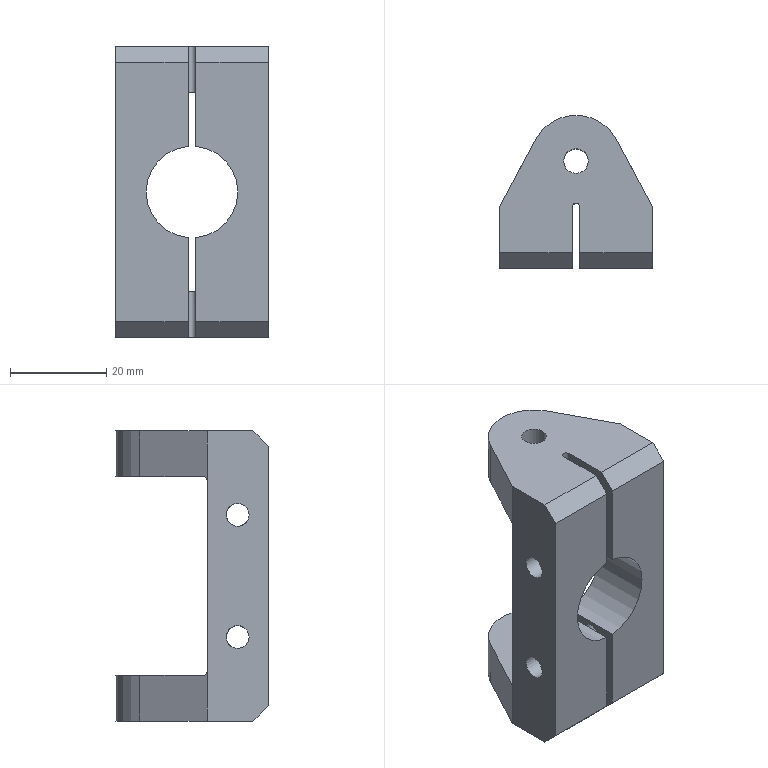Part | NX | features MG0330 trunion parts 24(stanchion group) 2 | 1 solid | 38 faces | box 31.75 x 31.75 x 60.325 mm | volume 25721 mm3 | plane 22 | cylinder 16 | commonest cylinder face diameters 1.524 x4 4.763 x4 19.05 x4 1.587 x2 5.105 x2
STEP:
#1=CARTESIAN_POINT('',(15.469,-15.113,-20.637));
#2=VERTEX_POINT('',#1);
#3=CARTESIAN_POINT('',(15.875,-15.875,-19.875));
#4=VERTEX_POINT('',#3);
#5=CARTESIAN_POINT('',(15.469,-15.113,-19.875));
#6=DIRECTION('',(0.8824,0.4706,0.));
#7=DIRECTION('',(0.4706,-0.8824,0.));
#8=AXIS2_PLACEMENT_3D('',#5,#6,#7);
#9=ELLIPSE('',#8,0.8636,0.762);
#10=EDGE_CURVE('',#2,#4,#9,.F.);
#11=ORIENTED_EDGE('',*,*,#10,.F.);
#12=CARTESIAN_POINT('',(0.2222,-15.113,-20.637));
#13=VERTEX_POINT('',#12);
#14=CARTESIAN_POINT('',(15.875,-15.113,-20.637));
#15=DIRECTION('',(-1.,0.,0.));
#16=VECTOR('',#15,1000.);
#17=LINE('',#14,#16);
#18=EDGE_CURVE('',#13,#2,#17,.F.);
#19=ORIENTED_EDGE('',*,*,#18,.F.);
#20=CARTESIAN_POINT('',(0.7937,-15.875,-19.875));
#21=VERTEX_POINT('',#20);
#22=CARTESIAN_POINT('',(0.2222,-15.113,-20.637));
#23=CARTESIAN_POINT('',(0.4532,-15.18,-20.637));
#24=CARTESIAN_POINT('',(0.8336,-15.592,-20.608));
#25=CARTESIAN_POINT('',(0.7937,-15.875,-20.117));
#26=CARTESIAN_POINT('',(0.7937,-15.875,-19.875));
#27=B_SPLINE_CURVE_WITH_KNOTS('',3,(#22,#23,#24,#25,#26),.UNSPECIFIED.,.F.,.F.,(4,1,4),(0.0004486,0.001169,0.001889),.UNSPECIFIED.);
#28=EDGE_CURVE('',#13,#21,#27,.T.);
#29=ORIENTED_EDGE('',*,*,#28,.T.);
#30=CARTESIAN_POINT('',(-15.875,-15.875,-19.875));
#31=DIRECTION('',(-1.,0.,0.));
#32=VECTOR('',#31,1000.);
#33=LINE('',#30,#32);
#34=EDGE_CURVE('',#4,#21,#33,.T.);
#35=ORIENTED_EDGE('',*,*,#34,.F.);
#36=EDGE_LOOP('',(#11,#19,#29,#35));
#37=FACE_BOUND('',#36,.T.);
#38=CARTESIAN_POINT('',(15.875,-15.113,-19.875));
#39=DIRECTION('',(1.,0.,0.));
#40=DIRECTION('',(0.,0.,-1.));
#41=AXIS2_PLACEMENT_3D('',#38,#39,#40);
#42=CYLINDRICAL_SURFACE('',#41,0.762);
#43=ADVANCED_FACE('',(#37),#42,.F.);
#44=CARTESIAN_POINT('',(0.,-8.903,-30.163));
#45=VERTEX_POINT('',#44);
#46=CARTESIAN_POINT('',(0.,-6.35,-30.163));
#47=DIRECTION('',(0.,0.,1.));
#48=DIRECTION('',(0.,-1.,0.));
#49=AXIS2_PLACEMENT_3D('',#46,#47,#48);
#50=CIRCLE('',#49,2.553);
#51=EDGE_CURVE('',#45,#45,#50,.T.);
#52=ORIENTED_EDGE('',*,*,#51,.T.);
#53=EDGE_LOOP('',(#52));
#54=FACE_BOUND('',#53,.T.);
#55=CARTESIAN_POINT('',(-8.404,-1.868,-30.163));
#56=VERTEX_POINT('',#55);
#57=CARTESIAN_POINT('',(-15.875,-15.875,-30.163));
#58=VERTEX_POINT('',#57);
#59=CARTESIAN_POINT('',(-0.9338,12.14,-30.163));
#60=DIRECTION('',(-0.4706,-0.8824,0.));
#61=VECTOR('',#60,1000.);
#62=LINE('',#59,#61);
#63=EDGE_CURVE('',#56,#58,#62,.T.);
#64=ORIENTED_EDGE('',*,*,#63,.F.);
#65=CARTESIAN_POINT('',(8.404,-1.868,-30.163));
#66=VERTEX_POINT('',#65);
#67=CARTESIAN_POINT('',(0.,-6.35,-30.163));
#68=DIRECTION('',(0.,0.,1.));
#69=DIRECTION('',(0.,-1.,0.));
#70=AXIS2_PLACEMENT_3D('',#67,#68,#69);
#71=CIRCLE('',#70,9.525);
#72=EDGE_CURVE('',#66,#56,#71,.T.);
#73=ORIENTED_EDGE('',*,*,#72,.F.);
#74=CARTESIAN_POINT('',(15.875,-15.875,-30.163));
#75=VERTEX_POINT('',#74);
#76=CARTESIAN_POINT('',(7.965,-1.044,-30.163));
#77=DIRECTION('',(-0.4706,0.8824,0.));
#78=VECTOR('',#77,1000.);
#79=LINE('',#76,#78);
#80=EDGE_CURVE('',#75,#66,#79,.T.);
#81=ORIENTED_EDGE('',*,*,#80,.F.);
#82=CARTESIAN_POINT('',(15.875,-25.4,-30.163));
#83=VERTEX_POINT('',#82);
#84=CARTESIAN_POINT('',(15.875,3.175,-30.163));
#85=DIRECTION('',(0.,1.,0.));
#86=VECTOR('',#85,1000.);
#87=LINE('',#84,#86);
#88=EDGE_CURVE('',#83,#75,#87,.T.);
#89=ORIENTED_EDGE('',*,*,#88,.F.);
#90=CARTESIAN_POINT('',(0.7937,-25.4,-30.163));
#91=VERTEX_POINT('',#90);
#92=CARTESIAN_POINT('',(15.875,-25.4,-30.163));
#93=DIRECTION('',(-1.,0.,0.));
#94=VECTOR('',#93,1000.);
#95=LINE('',#92,#94);
#96=EDGE_CURVE('',#83,#91,#95,.T.);
#97=ORIENTED_EDGE('',*,*,#96,.T.);
#98=CARTESIAN_POINT('',(0.7937,-15.875,-30.163));
#99=VERTEX_POINT('',#98);
#100=CARTESIAN_POINT('',(0.7937,3.175,-30.163));
#101=DIRECTION('',(0.,1.,0.));
#102=VECTOR('',#101,1000.);
#103=LINE('',#100,#102);
#104=EDGE_CURVE('',#91,#99,#103,.T.);
#105=ORIENTED_EDGE('',*,*,#104,.T.);
#106=CARTESIAN_POINT('',(-0.7937,-15.875,-30.163));
#107=VERTEX_POINT('',#106);
#108=CARTESIAN_POINT('',(0.,-15.875,-30.163));
#109=DIRECTION('',(0.,0.,1.));
#110=DIRECTION('',(0.,-1.,0.));
#111=AXIS2_PLACEMENT_3D('',#108,#109,#110);
#112=CIRCLE('',#111,0.7937);
#113=EDGE_CURVE('',#99,#107,#112,.T.);
#114=ORIENTED_EDGE('',*,*,#113,.T.);
#115=CARTESIAN_POINT('',(-0.7937,-25.4,-30.163));
#116=VERTEX_POINT('',#115);
#117=CARTESIAN_POINT('',(-0.7937,3.175,-30.163));
#118=DIRECTION('',(0.,-1.,0.));
#119=VECTOR('',#118,1000.);
#120=LINE('',#117,#119);
#121=EDGE_CURVE('',#107,#116,#120,.T.);
#122=ORIENTED_EDGE('',*,*,#121,.T.);
#123=CARTESIAN_POINT('',(-15.875,-25.4,-30.163));
#124=VERTEX_POINT('',#123);
#125=CARTESIAN_POINT('',(15.875,-25.4,-30.163));
#126=DIRECTION('',(-1.,0.,0.));
#127=VECTOR('',#126,1000.);
#128=LINE('',#125,#127);
#129=EDGE_CURVE('',#116,#124,#128,.T.);
#130=ORIENTED_EDGE('',*,*,#129,.T.);
#131=CARTESIAN_POINT('',(-15.875,3.175,-30.163));
#132=DIRECTION('',(0.,1.,0.));
#133=VECTOR('',#132,1000.);
#134=LINE('',#131,#133);
#135=EDGE_CURVE('',#124,#58,#134,.T.);
#136=ORIENTED_EDGE('',*,*,#135,.T.);
#137=EDGE_LOOP('',(#64,#73,#81,#89,#97,#105,#114,#122,#130,#136));
#138=FACE_BOUND('',#137,.T.);
#139=CARTESIAN_POINT('',(15.875,3.175,-30.163));
#140=DIRECTION('',(0.,0.,1.));
#141=DIRECTION('',(0.,-1.,0.));
#142=AXIS2_PLACEMENT_3D('',#139,#140,#141);
#143=PLANE('',#142);
#144=ADVANCED_FACE('',(#54,#138),#143,.F.);
#145=CARTESIAN_POINT('',(0.,-3.797,-20.637));
#146=VERTEX_POINT('',#145);
#147=CARTESIAN_POINT('',(0.,-6.35,-20.637));
#148=DIRECTION('',(0.,0.,-1.));
#149=DIRECTION('',(0.,1.,0.));
#150=AXIS2_PLACEMENT_3D('',#147,#148,#149);
#151=CIRCLE('',#150,2.553);
#152=EDGE_CURVE('',#146,#146,#151,.T.);
#153=ORIENTED_EDGE('',*,*,#152,.T.);
#154=EDGE_LOOP('',(#153));
#155=FACE_BOUND('',#154,.T.);
#156=CARTESIAN_POINT('',(-15.469,-15.113,-20.637));
#157=VERTEX_POINT('',#156);
#158=CARTESIAN_POINT('',(-8.404,-1.868,-20.637));
#159=VERTEX_POINT('',#158);
#160=CARTESIAN_POINT('',(-0.9338,12.14,-20.637));
#161=DIRECTION('',(0.4706,0.8824,0.));
#162=VECTOR('',#161,1000.);
#163=LINE('',#160,#162);
#164=EDGE_CURVE('',#157,#159,#163,.T.);
#165=ORIENTED_EDGE('',*,*,#164,.F.);
#166=CARTESIAN_POINT('',(-0.2222,-15.113,-20.637));
#167=VERTEX_POINT('',#166);
#168=CARTESIAN_POINT('',(15.875,-15.113,-20.637));
#169=DIRECTION('',(-1.,0.,0.));
#170=VECTOR('',#169,1000.);
#171=LINE('',#168,#170);
#172=EDGE_CURVE('',#157,#167,#171,.F.);
#173=ORIENTED_EDGE('',*,*,#172,.T.);
#174=CARTESIAN_POINT('',(0.,-15.875,-20.637));
#175=DIRECTION('',(0.,0.,-1.));
#176=DIRECTION('',(0.,1.,0.));
#177=AXIS2_PLACEMENT_3D('',#174,#175,#176);
#178=CIRCLE('',#177,0.7937);
#179=EDGE_CURVE('',#167,#13,#178,.T.);
#180=ORIENTED_EDGE('',*,*,#179,.T.);
#181=ORIENTED_EDGE('',*,*,#18,.T.);
#182=CARTESIAN_POINT('',(8.404,-1.868,-20.637));
#183=VERTEX_POINT('',#182);
#184=CARTESIAN_POINT('',(7.965,-1.044,-20.637));
#185=DIRECTION('',(0.4706,-0.8824,0.));
#186=VECTOR('',#185,1000.);
#187=LINE('',#184,#186);
#188=EDGE_CURVE('',#183,#2,#187,.T.);
#189=ORIENTED_EDGE('',*,*,#188,.F.);
#190=CARTESIAN_POINT('',(0.,-6.35,-20.637));
#191=DIRECTION('',(0.,0.,-1.));
#192=DIRECTION('',(0.,1.,0.));
#193=AXIS2_PLACEMENT_3D('',#190,#191,#192);
#194=CIRCLE('',#193,9.525);
#195=EDGE_CURVE('',#159,#183,#194,.T.);
#196=ORIENTED_EDGE('',*,*,#195,.F.);
#197=EDGE_LOOP('',(#165,#173,#180,#181,#189,#196));
#198=FACE_BOUND('',#197,.T.);
#199=CARTESIAN_POINT('',(15.875,3.175,-20.637));
#200=DIRECTION('',(0.,0.,-1.));
#201=DIRECTION('',(0.,1.,0.));
#202=AXIS2_PLACEMENT_3D('',#199,#200,#201);
#203=PLANE('',#202);
#204=ADVANCED_FACE('',(#155,#198),#203,.F.);
#205=CARTESIAN_POINT('',(15.875,-22.225,15.081));
#206=VERTEX_POINT('',#205);
#207=CARTESIAN_POINT('',(15.875,-22.225,12.7));
#208=DIRECTION('',(-1.,0.,0.));
#209=DIRECTION('',(0.,0.,1.));
#210=AXIS2_PLACEMENT_3D('',#207,#208,#209);
#211=CIRCLE('',#210,2.381);
#212=EDGE_CURVE('',#206,#206,#211,.T.);
#213=ORIENTED_EDGE('',*,*,#212,.T.);
#214=EDGE_LOOP('',(#213));
#215=FACE_BOUND('',#214,.T.);
#216=CARTESIAN_POINT('',(15.875,-22.225,-10.319));
#217=VERTEX_POINT('',#216);
#218=CARTESIAN_POINT('',(15.875,-22.225,-12.7));
#219=DIRECTION('',(-1.,0.,0.));
#220=DIRECTION('',(0.,0.,1.));
#221=AXIS2_PLACEMENT_3D('',#218,#219,#220);
#222=CIRCLE('',#221,2.381);
#223=EDGE_CURVE('',#217,#217,#222,.T.);
#224=ORIENTED_EDGE('',*,*,#223,.T.);
#225=EDGE_LOOP('',(#224));
#226=FACE_BOUND('',#225,.T.);
#227=CARTESIAN_POINT('',(15.875,-15.875,30.163));
#228=VERTEX_POINT('',#227);
#229=CARTESIAN_POINT('',(15.875,-15.875,19.875));
#230=VERTEX_POINT('',#229);
#231=CARTESIAN_POINT('',(15.875,-15.875,494.417));
#232=DIRECTION('',(0.,0.,-1.));
#233=VECTOR('',#232,1000.);
#234=LINE('',#231,#233);
#235=EDGE_CURVE('',#228,#230,#234,.T.);
#236=ORIENTED_EDGE('',*,*,#235,.F.);
#237=CARTESIAN_POINT('',(15.875,-25.4,30.163));
#238=VERTEX_POINT('',#237);
#239=CARTESIAN_POINT('',(15.875,3.175,30.163));
#240=DIRECTION('',(0.,1.,0.));
#241=VECTOR('',#240,1000.);
#242=LINE('',#239,#241);
#243=EDGE_CURVE('',#238,#228,#242,.T.);
#244=ORIENTED_EDGE('',*,*,#243,.F.);
#245=CARTESIAN_POINT('',(15.875,-28.575,26.988));
#246=VERTEX_POINT('',#245);
#247=CARTESIAN_POINT('',(15.875,-25.4,30.163));
#248=DIRECTION('',(0.,-0.7071,-0.7071));
#249=VECTOR('',#248,1000.);
#250=LINE('',#247,#249);
#251=EDGE_CURVE('',#246,#238,#250,.F.);
#252=ORIENTED_EDGE('',*,*,#251,.F.);
#253=CARTESIAN_POINT('',(15.875,-28.575,-26.988));
#254=VERTEX_POINT('',#253);
#255=CARTESIAN_POINT('',(15.875,-28.575,-30.163));
#256=DIRECTION('',(0.,0.,-1.));
#257=VECTOR('',#256,1000.);
#258=LINE('',#255,#257);
#259=EDGE_CURVE('',#246,#254,#258,.T.);
#260=ORIENTED_EDGE('',*,*,#259,.T.);
#261=CARTESIAN_POINT('',(15.875,-25.4,-30.163));
#262=DIRECTION('',(0.,-0.7071,0.7071));
#263=VECTOR('',#262,1000.);
#264=LINE('',#261,#263);
#265=EDGE_CURVE('',#254,#83,#264,.F.);
#266=ORIENTED_EDGE('',*,*,#265,.T.);
#267=ORIENTED_EDGE('',*,*,#88,.T.);
#268=CARTESIAN_POINT('',(15.875,-15.875,494.417));
#269=DIRECTION('',(0.,0.,-1.));
#270=VECTOR('',#269,1000.);
#271=LINE('',#268,#270);
#272=EDGE_CURVE('',#4,#75,#271,.T.);
#273=ORIENTED_EDGE('',*,*,#272,.F.);
#274=CARTESIAN_POINT('',(15.875,-15.875,-20.637));
#275=DIRECTION('',(0.,0.,1.));
#276=VECTOR('',#275,1000.);
#277=LINE('',#274,#276);
#278=EDGE_CURVE('',#4,#230,#277,.T.);
#279=ORIENTED_EDGE('',*,*,#278,.T.);
#280=EDGE_LOOP('',(#236,#244,#252,#260,#266,#267,#273,#279));
#281=FACE_BOUND('',#280,.T.);
#282=CARTESIAN_POINT('',(15.875,-28.575,-30.163));
#283=DIRECTION('',(-1.,0.,0.));
#284=DIRECTION('',(0.,0.,1.));
#285=AXIS2_PLACEMENT_3D('',#282,#283,#284);
#286=PLANE('',#285);
#287=ADVANCED_FACE('',(#215,#226,#281),#286,.F.);
#288=CARTESIAN_POINT('',(-15.875,-22.225,15.081));
#289=VERTEX_POINT('',#288);
#290=CARTESIAN_POINT('',(-15.875,-22.225,12.7));
#291=DIRECTION('',(-1.,0.,0.));
#292=DIRECTION('',(0.,0.,1.));
#293=AXIS2_PLACEMENT_3D('',#290,#291,#292);
#294=CIRCLE('',#293,2.381);
#295=EDGE_CURVE('',#289,#289,#294,.F.);
#296=ORIENTED_EDGE('',*,*,#295,.T.);
#297=EDGE_LOOP('',(#296));
#298=FACE_BOUND('',#297,.T.);
#299=CARTESIAN_POINT('',(-15.875,-22.225,-10.319));
#300=VERTEX_POINT('',#299);
#301=CARTESIAN_POINT('',(-15.875,-22.225,-12.7));
#302=DIRECTION('',(-1.,0.,0.));
#303=DIRECTION('',(0.,0.,1.));
#304=AXIS2_PLACEMENT_3D('',#301,#302,#303);
#305=CIRCLE('',#304,2.381);
#306=EDGE_CURVE('',#300,#300,#305,.F.);
#307=ORIENTED_EDGE('',*,*,#306,.T.);
#308=EDGE_LOOP('',(#307));
#309=FACE_BOUND('',#308,.T.);
#310=CARTESIAN_POINT('',(-15.875,-25.4,30.163));
#311=VERTEX_POINT('',#310);
#312=CARTESIAN_POINT('',(-15.875,-15.875,30.163));
#313=VERTEX_POINT('',#312);
#314=CARTESIAN_POINT('',(-15.875,3.175,30.163));
#315=DIRECTION('',(0.,1.,0.));
#316=VECTOR('',#315,1000.);
#317=LINE('',#314,#316);
#318=EDGE_CURVE('',#311,#313,#317,.T.);
#319=ORIENTED_EDGE('',*,*,#318,.T.);
#320=CARTESIAN_POINT('',(-15.875,-15.875,19.875));
#321=VERTEX_POINT('',#320);
#322=CARTESIAN_POINT('',(-15.875,-15.875,494.417));
#323=DIRECTION('',(0.,0.,-1.));
#324=VECTOR('',#323,1000.);
#325=LINE('',#322,#324);
#326=EDGE_CURVE('',#313,#321,#325,.T.);
#327=ORIENTED_EDGE('',*,*,#326,.T.);
#328=CARTESIAN_POINT('',(-15.875,-15.875,-19.875));
#329=VERTEX_POINT('',#328);
#330=CARTESIAN_POINT('',(-15.875,-15.875,-20.637));
#331=DIRECTION('',(0.,0.,1.));
#332=VECTOR('',#331,1000.);
#333=LINE('',#330,#332);
#334=EDGE_CURVE('',#329,#321,#333,.T.);
#335=ORIENTED_EDGE('',*,*,#334,.F.);
#336=CARTESIAN_POINT('',(-15.875,-15.875,494.417));
#337=DIRECTION('',(0.,0.,-1.));
#338=VECTOR('',#337,1000.);
#339=LINE('',#336,#338);
#340=EDGE_CURVE('',#329,#58,#339,.T.);
#341=ORIENTED_EDGE('',*,*,#340,.T.);
#342=ORIENTED_EDGE('',*,*,#135,.F.);
#343=CARTESIAN_POINT('',(-15.875,-28.575,-26.988));
#344=VERTEX_POINT('',#343);
#345=CARTESIAN_POINT('',(-15.875,-26.988,-28.575));
#346=DIRECTION('',(0.,0.7071,-0.7071));
#347=VECTOR('',#346,1000.);
#348=LINE('',#345,#347);
#349=EDGE_CURVE('',#124,#344,#348,.F.);
#350=ORIENTED_EDGE('',*,*,#349,.T.);
#351=CARTESIAN_POINT('',(-15.875,-28.575,26.988));
#352=VERTEX_POINT('',#351);
#353=CARTESIAN_POINT('',(-15.875,-28.575,-30.163));
#354=DIRECTION('',(0.,0.,-1.));
#355=VECTOR('',#354,1000.);
#356=LINE('',#353,#355);
#357=EDGE_CURVE('',#352,#344,#356,.T.);
#358=ORIENTED_EDGE('',*,*,#357,.F.);
#359=CARTESIAN_POINT('',(-15.875,-26.988,28.575));
#360=DIRECTION('',(0.,0.7071,0.7071));
#361=VECTOR('',#360,1000.);
#362=LINE('',#359,#361);
#363=EDGE_CURVE('',#311,#352,#362,.F.);
#364=ORIENTED_EDGE('',*,*,#363,.F.);
#365=EDGE_LOOP('',(#319,#327,#335,#341,#342,#350,#358,#364));
#366=FACE_BOUND('',#365,.T.);
#367=CARTESIAN_POINT('',(-15.875,-28.575,-30.163));
#368=DIRECTION('',(-1.,0.,0.));
#369=DIRECTION('',(0.,0.,1.));
#370=AXIS2_PLACEMENT_3D('',#367,#368,#369);
#371=PLANE('',#370);
#372=ADVANCED_FACE('',(#298,#309,#366),#371,.T.);
#373=CARTESIAN_POINT('',(-15.469,-15.113,-19.875));
#374=DIRECTION('',(-0.8824,0.4706,0.));
#375=DIRECTION('',(0.4706,0.8824,0.));
#376=AXIS2_PLACEMENT_3D('',#373,#374,#375);
#377=ELLIPSE('',#376,0.8636,0.762);
#378=EDGE_CURVE('',#329,#157,#377,.F.);
#379=ORIENTED_EDGE('',*,*,#378,.F.);
#380=CARTESIAN_POINT('',(-0.7937,-15.875,-19.875));
#381=VERTEX_POINT('',#380);
#382=CARTESIAN_POINT('',(-15.875,-15.875,-19.875));
#383=DIRECTION('',(-1.,0.,0.));
#384=VECTOR('',#383,1000.);
#385=LINE('',#382,#384);
#386=EDGE_CURVE('',#381,#329,#385,.T.);
#387=ORIENTED_EDGE('',*,*,#386,.F.);
#388=CARTESIAN_POINT('',(-0.7938,-15.875,-19.875));
#389=CARTESIAN_POINT('',(-0.7938,-15.875,-20.118));
#390=CARTESIAN_POINT('',(-0.834,-15.595,-20.605));
#391=CARTESIAN_POINT('',(-0.4553,-15.181,-20.637));
#392=CARTESIAN_POINT('',(-0.2222,-15.113,-20.637));
#393=B_SPLINE_CURVE_WITH_KNOTS('',3,(#388,#389,#390,#391,#392),.UNSPECIFIED.,.F.,.F.,(4,1,4),(0.005213,0.005931,0.006649),.UNSPECIFIED.);
#394=EDGE_CURVE('',#381,#167,#393,.T.);
#395=ORIENTED_EDGE('',*,*,#394,.T.);
#396=ORIENTED_EDGE('',*,*,#172,.F.);
#397=EDGE_LOOP('',(#379,#387,#395,#396));
#398=FACE_BOUND('',#397,.T.);
#399=CARTESIAN_POINT('',(15.875,-15.113,-19.875));
#400=DIRECTION('',(1.,0.,0.));
#401=DIRECTION('',(0.,0.,-1.));
#402=AXIS2_PLACEMENT_3D('',#399,#400,#401);
#403=CYLINDRICAL_SURFACE('',#402,0.762);
#404=ADVANCED_FACE('',(#398),#403,.F.);
#405=CARTESIAN_POINT('',(15.469,-15.113,20.637));
#406=VERTEX_POINT('',#405);
#407=CARTESIAN_POINT('',(15.469,-15.113,19.875));
#408=DIRECTION('',(0.8824,0.4706,0.));
#409=DIRECTION('',(0.4706,-0.8824,0.));
#410=AXIS2_PLACEMENT_3D('',#407,#408,#409);
#411=ELLIPSE('',#410,0.8636,0.762);
#412=EDGE_CURVE('',#230,#406,#411,.F.);
#413=ORIENTED_EDGE('',*,*,#412,.F.);
#414=CARTESIAN_POINT('',(0.7937,-15.875,19.875));
#415=VERTEX_POINT('',#414);
#416=CARTESIAN_POINT('',(-15.875,-15.875,19.875));
#417=DIRECTION('',(-1.,0.,0.));
#418=VECTOR('',#417,1000.);
#419=LINE('',#416,#418);
#420=EDGE_CURVE('',#230,#415,#419,.T.);
#421=ORIENTED_EDGE('',*,*,#420,.T.);
#422=CARTESIAN_POINT('',(0.2222,-15.113,20.637));
#423=VERTEX_POINT('',#422);
#424=CARTESIAN_POINT('',(0.2222,-15.113,20.637));
#425=CARTESIAN_POINT('',(0.4532,-15.18,20.637));
#426=CARTESIAN_POINT('',(0.8336,-15.592,20.608));
#427=CARTESIAN_POINT('',(0.7937,-15.875,20.117));
#428=CARTESIAN_POINT('',(0.7937,-15.875,19.875));
#429=B_SPLINE_CURVE_WITH_KNOTS('',3,(#424,#425,#426,#427,#428),.UNSPECIFIED.,.F.,.F.,(4,1,4),(0.0004486,0.001169,0.001889),.UNSPECIFIED.);
#430=EDGE_CURVE('',#423,#415,#429,.T.);
#431=ORIENTED_EDGE('',*,*,#430,.F.);
#432=CARTESIAN_POINT('',(15.875,-15.113,20.637));
#433=DIRECTION('',(-1.,0.,0.));
#434=VECTOR('',#433,1000.);
#435=LINE('',#432,#434);
#436=EDGE_CURVE('',#423,#406,#435,.F.);
#437=ORIENTED_EDGE('',*,*,#436,.T.);
#438=EDGE_LOOP('',(#413,#421,#431,#437));
#439=FACE_BOUND('',#438,.T.);
#440=CARTESIAN_POINT('',(15.875,-15.113,19.875));
#441=DIRECTION('',(1.,0.,0.));
#442=DIRECTION('',(0.,0.,1.));
#443=AXIS2_PLACEMENT_3D('',#440,#441,#442);
#444=CYLINDRICAL_SURFACE('',#443,0.762);
#445=ADVANCED_FACE('',(#439),#444,.F.);
#446=CARTESIAN_POINT('',(0.,-3.797,30.163));
#447=VERTEX_POINT('',#446);
#448=CARTESIAN_POINT('',(0.,-6.35,30.163));
#449=DIRECTION('',(0.,0.,-1.));
#450=DIRECTION('',(0.,1.,0.));
#451=AXIS2_PLACEMENT_3D('',#448,#449,#450);
#452=CIRCLE('',#451,2.553);
#453=EDGE_CURVE('',#447,#447,#452,.F.);
#454=ORIENTED_EDGE('',*,*,#453,.F.);
#455=EDGE_LOOP('',(#454));
#456=FACE_BOUND('',#455,.T.);
#457=CARTESIAN_POINT('',(-8.404,-1.868,30.163));
#458=VERTEX_POINT('',#457);
#459=CARTESIAN_POINT('',(-0.9338,12.14,30.163));
#460=DIRECTION('',(0.4706,0.8824,0.));
#461=VECTOR('',#460,1000.);
#462=LINE('',#459,#461);
#463=EDGE_CURVE('',#313,#458,#462,.T.);
#464=ORIENTED_EDGE('',*,*,#463,.F.);
#465=ORIENTED_EDGE('',*,*,#318,.F.);
#466=CARTESIAN_POINT('',(-0.7937,-25.4,30.163));
#467=VERTEX_POINT('',#466);
#468=CARTESIAN_POINT('',(15.875,-25.4,30.163));
#469=DIRECTION('',(-1.,0.,0.));
#470=VECTOR('',#469,1000.);
#471=LINE('',#468,#470);
#472=EDGE_CURVE('',#467,#311,#471,.T.);
#473=ORIENTED_EDGE('',*,*,#472,.F.);
#474=CARTESIAN_POINT('',(-0.7937,-15.875,30.163));
#475=VERTEX_POINT('',#474);
#476=CARTESIAN_POINT('',(-0.7937,3.175,30.163));
#477=DIRECTION('',(0.,-1.,0.));
#478=VECTOR('',#477,1000.);
#479=LINE('',#476,#478);
#480=EDGE_CURVE('',#475,#467,#479,.T.);
#481=ORIENTED_EDGE('',*,*,#480,.F.);
#482=CARTESIAN_POINT('',(0.7937,-15.875,30.163));
#483=VERTEX_POINT('',#482);
#484=CARTESIAN_POINT('',(0.,-15.875,30.163));
#485=DIRECTION('',(0.,0.,1.));
#486=DIRECTION('',(0.,-1.,0.));
#487=AXIS2_PLACEMENT_3D('',#484,#485,#486);
#488=CIRCLE('',#487,0.7937);
#489=EDGE_CURVE('',#483,#475,#488,.T.);
#490=ORIENTED_EDGE('',*,*,#489,.F.);
#491=CARTESIAN_POINT('',(0.7937,-25.4,30.163));
#492=VERTEX_POINT('',#491);
#493=CARTESIAN_POINT('',(0.7937,3.175,30.163));
#494=DIRECTION('',(0.,1.,0.));
#495=VECTOR('',#494,1000.);
#496=LINE('',#493,#495);
#497=EDGE_CURVE('',#492,#483,#496,.T.);
#498=ORIENTED_EDGE('',*,*,#497,.F.);
#499=CARTESIAN_POINT('',(15.875,-25.4,30.163));
#500=DIRECTION('',(-1.,0.,0.));
#501=VECTOR('',#500,1000.);
#502=LINE('',#499,#501);
#503=EDGE_CURVE('',#238,#492,#502,.T.);
#504=ORIENTED_EDGE('',*,*,#503,.F.);
#505=ORIENTED_EDGE('',*,*,#243,.T.);
#506=CARTESIAN_POINT('',(8.404,-1.868,30.163));
#507=VERTEX_POINT('',#506);
#508=CARTESIAN_POINT('',(7.965,-1.044,30.163));
#509=DIRECTION('',(0.4706,-0.8824,0.));
#510=VECTOR('',#509,1000.);
#511=LINE('',#508,#510);
#512=EDGE_CURVE('',#507,#228,#511,.T.);
#513=ORIENTED_EDGE('',*,*,#512,.F.);
#514=CARTESIAN_POINT('',(0.,-6.35,30.163));
#515=DIRECTION('',(0.,0.,-1.));
#516=DIRECTION('',(0.,1.,0.));
#517=AXIS2_PLACEMENT_3D('',#514,#515,#516);
#518=CIRCLE('',#517,9.525);
#519=EDGE_CURVE('',#458,#507,#518,.T.);
#520=ORIENTED_EDGE('',*,*,#519,.F.);
#521=EDGE_LOOP('',(#464,#465,#473,#481,#490,#498,#504,#505,#513,#520));
#522=FACE_BOUND('',#521,.T.);
#523=CARTESIAN_POINT('',(15.875,3.175,30.163));
#524=DIRECTION('',(0.,0.,-1.));
#525=DIRECTION('',(0.,-1.,0.));
#526=AXIS2_PLACEMENT_3D('',#523,#524,#525);
#527=PLANE('',#526);
#528=ADVANCED_FACE('',(#456,#522),#527,.F.);
#529=CARTESIAN_POINT('',(0.,-8.903,20.637));
#530=VERTEX_POINT('',#529);
#531=CARTESIAN_POINT('',(0.,-6.35,20.637));
#532=DIRECTION('',(0.,0.,1.));
#533=DIRECTION('',(0.,-1.,0.));
#534=AXIS2_PLACEMENT_3D('',#531,#532,#533);
#535=CIRCLE('',#534,2.553);
#536=EDGE_CURVE('',#530,#530,#535,.F.);
#537=ORIENTED_EDGE('',*,*,#536,.F.);
#538=EDGE_LOOP('',(#537));
#539=FACE_BOUND('',#538,.T.);
#540=CARTESIAN_POINT('',(-8.404,-1.868,20.637));
#541=VERTEX_POINT('',#540);
#542=CARTESIAN_POINT('',(-15.469,-15.113,20.637));
#543=VERTEX_POINT('',#542);
#544=CARTESIAN_POINT('',(-0.9338,12.14,20.637));
#545=DIRECTION('',(-0.4706,-0.8824,0.));
#546=VECTOR('',#545,1000.);
#547=LINE('',#544,#546);
#548=EDGE_CURVE('',#541,#543,#547,.T.);
#549=ORIENTED_EDGE('',*,*,#548,.F.);
#550=CARTESIAN_POINT('',(8.404,-1.868,20.637));
#551=VERTEX_POINT('',#550);
#552=CARTESIAN_POINT('',(0.,-6.35,20.637));
#553=DIRECTION('',(0.,0.,1.));
#554=DIRECTION('',(0.,-1.,0.));
#555=AXIS2_PLACEMENT_3D('',#552,#553,#554);
#556=CIRCLE('',#555,9.525);
#557=EDGE_CURVE('',#551,#541,#556,.T.);
#558=ORIENTED_EDGE('',*,*,#557,.F.);
#559=CARTESIAN_POINT('',(7.965,-1.044,20.637));
#560=DIRECTION('',(-0.4706,0.8824,0.));
#561=VECTOR('',#560,1000.);
#562=LINE('',#559,#561);
#563=EDGE_CURVE('',#406,#551,#562,.T.);
#564=ORIENTED_EDGE('',*,*,#563,.F.);
#565=ORIENTED_EDGE('',*,*,#436,.F.);
#566=CARTESIAN_POINT('',(-0.2222,-15.113,20.637));
#567=VERTEX_POINT('',#566);
#568=CARTESIAN_POINT('',(0.,-15.875,20.637));
#569=DIRECTION('',(0.,0.,-1.));
#570=DIRECTION('',(0.,1.,0.));
#571=AXIS2_PLACEMENT_3D('',#568,#569,#570);
#572=CIRCLE('',#571,0.7937);
#573=EDGE_CURVE('',#567,#423,#572,.T.);
#574=ORIENTED_EDGE('',*,*,#573,.F.);
#575=CARTESIAN_POINT('',(15.875,-15.113,20.637));
#576=DIRECTION('',(-1.,0.,0.));
#577=VECTOR('',#576,1000.);
#578=LINE('',#575,#577);
#579=EDGE_CURVE('',#543,#567,#578,.F.);
#580=ORIENTED_EDGE('',*,*,#579,.F.);
#581=EDGE_LOOP('',(#549,#558,#564,#565,#574,#580));
#582=FACE_BOUND('',#581,.T.);
#583=CARTESIAN_POINT('',(15.875,3.175,20.637));
#584=DIRECTION('',(0.,0.,1.));
#585=DIRECTION('',(0.,1.,0.));
#586=AXIS2_PLACEMENT_3D('',#583,#584,#585);
#587=PLANE('',#586);
#588=ADVANCED_FACE('',(#539,#582),#587,.F.);
#589=CARTESIAN_POINT('',(-15.469,-15.113,19.875));
#590=DIRECTION('',(-0.8824,0.4706,0.));
#591=DIRECTION('',(0.4706,0.8824,0.));
#592=AXIS2_PLACEMENT_3D('',#589,#590,#591);
#593=ELLIPSE('',#592,0.8636,0.762);
#594=EDGE_CURVE('',#543,#321,#593,.F.);
#595=ORIENTED_EDGE('',*,*,#594,.F.);
#596=ORIENTED_EDGE('',*,*,#579,.T.);
#597=CARTESIAN_POINT('',(-0.7937,-15.875,19.875));
#598=VERTEX_POINT('',#597);
#599=CARTESIAN_POINT('',(-0.7938,-15.875,19.875));
#600=CARTESIAN_POINT('',(-0.7938,-15.875,20.118));
#601=CARTESIAN_POINT('',(-0.834,-15.595,20.605));
#602=CARTESIAN_POINT('',(-0.4553,-15.181,20.637));
#603=CARTESIAN_POINT('',(-0.2222,-15.113,20.637));
#604=B_SPLINE_CURVE_WITH_KNOTS('',3,(#599,#600,#601,#602,#603),.UNSPECIFIED.,.F.,.F.,(4,1,4),(0.005213,0.005931,0.006649),.UNSPECIFIED.);
#605=EDGE_CURVE('',#598,#567,#604,.T.);
#606=ORIENTED_EDGE('',*,*,#605,.F.);
#607=CARTESIAN_POINT('',(-15.875,-15.875,19.875));
#608=DIRECTION('',(-1.,0.,0.));
#609=VECTOR('',#608,1000.);
#610=LINE('',#607,#609);
#611=EDGE_CURVE('',#598,#321,#610,.T.);
#612=ORIENTED_EDGE('',*,*,#611,.T.);
#613=EDGE_LOOP('',(#595,#596,#606,#612));
#614=FACE_BOUND('',#613,.T.);
#615=CARTESIAN_POINT('',(15.875,-15.113,19.875));
#616=DIRECTION('',(1.,0.,0.));
#617=DIRECTION('',(0.,0.,1.));
#618=AXIS2_PLACEMENT_3D('',#615,#616,#617);
#619=CYLINDRICAL_SURFACE('',#618,0.762);
#620=ADVANCED_FACE('',(#614),#619,.F.);
#621=CARTESIAN_POINT('',(0.7937,-19.844,-12.7));
#622=VERTEX_POINT('',#621);
#623=CARTESIAN_POINT('',(0.7937,-22.225,-12.7));
#624=DIRECTION('',(1.,0.,0.));
#625=DIRECTION('',(0.,1.,0.));
#626=AXIS2_PLACEMENT_3D('',#623,#624,#625);
#627=CIRCLE('',#626,2.381);
#628=EDGE_CURVE('',#622,#622,#627,.T.);
#629=ORIENTED_EDGE('',*,*,#628,.T.);
#630=EDGE_LOOP('',(#629));
#631=FACE_BOUND('',#630,.T.);
#632=CARTESIAN_POINT('',(0.7937,-28.575,-26.988));
#633=VERTEX_POINT('',#632);
#634=CARTESIAN_POINT('',(0.7937,-28.575,-9.492));
#635=VERTEX_POINT('',#634);
#636=CARTESIAN_POINT('',(0.7937,-28.575,-34.925));
#637=DIRECTION('',(0.,0.,1.));
#638=VECTOR('',#637,1000.);
#639=LINE('',#636,#638);
#640=EDGE_CURVE('',#633,#635,#639,.T.);
#641=ORIENTED_EDGE('',*,*,#640,.T.);
#642=CARTESIAN_POINT('',(0.7937,-15.875,-9.492));
#643=VERTEX_POINT('',#642);
#644=CARTESIAN_POINT('',(0.7937,-55.516,-9.492));
#645=DIRECTION('',(0.,1.,0.));
#646=VECTOR('',#645,1000.);
#647=LINE('',#644,#646);
#648=EDGE_CURVE('',#635,#643,#647,.T.);
#649=ORIENTED_EDGE('',*,*,#648,.T.);
#650=CARTESIAN_POINT('',(0.7937,-15.875,-34.925));
#651=DIRECTION('',(0.,0.,1.));
#652=VECTOR('',#651,1000.);
#653=LINE('',#650,#652);
#654=EDGE_CURVE('',#21,#643,#653,.T.);
#655=ORIENTED_EDGE('',*,*,#654,.F.);
#656=CARTESIAN_POINT('',(0.7937,-15.875,-34.925));
#657=DIRECTION('',(0.,0.,1.));
#658=VECTOR('',#657,1000.);
#659=LINE('',#656,#658);
#660=EDGE_CURVE('',#99,#21,#659,.T.);
#661=ORIENTED_EDGE('',*,*,#660,.F.);
#662=ORIENTED_EDGE('',*,*,#104,.F.);
#663=CARTESIAN_POINT('',(0.7937,-25.4,-30.163));
#664=DIRECTION('',(0.,0.7071,-0.7071));
#665=VECTOR('',#664,1000.);
#666=LINE('',#663,#665);
#667=EDGE_CURVE('',#91,#633,#666,.F.);
#668=ORIENTED_EDGE('',*,*,#667,.T.);
#669=EDGE_LOOP('',(#641,#649,#655,#661,#662,#668));
#670=FACE_BOUND('',#669,.T.);
#671=CARTESIAN_POINT('',(0.7937,-28.575,-34.925));
#672=DIRECTION('',(1.,0.,0.));
#673=DIRECTION('',(0.,1.,0.));
#674=AXIS2_PLACEMENT_3D('',#671,#672,#673);
#675=PLANE('',#674);
#676=ADVANCED_FACE('',(#631,#670),#675,.F.);
#677=CARTESIAN_POINT('',(-0.7937,-24.606,12.7));
#678=VERTEX_POINT('',#677);
#679=CARTESIAN_POINT('',(-0.7937,-22.225,12.7));
#680=DIRECTION('',(-1.,0.,0.));
#681=DIRECTION('',(0.,-1.,0.));
#682=AXIS2_PLACEMENT_3D('',#679,#680,#681);
#683=CIRCLE('',#682,2.381);
#684=EDGE_CURVE('',#678,#678,#683,.T.);
#685=ORIENTED_EDGE('',*,*,#684,.T.);
#686=EDGE_LOOP('',(#685));
#687=FACE_BOUND('',#686,.T.);
#688=CARTESIAN_POINT('',(-0.7937,-28.575,9.492));
#689=VERTEX_POINT('',#688);
#690=CARTESIAN_POINT('',(-0.7937,-28.575,26.988));
#691=VERTEX_POINT('',#690);
#692=CARTESIAN_POINT('',(-0.7937,-28.575,-34.925));
#693=DIRECTION('',(0.,0.,1.));
#694=VECTOR('',#693,1000.);
#695=LINE('',#692,#694);
#696=EDGE_CURVE('',#689,#691,#695,.T.);
#697=ORIENTED_EDGE('',*,*,#696,.F.);
#698=CARTESIAN_POINT('',(-0.7937,-15.875,9.492));
#699=VERTEX_POINT('',#698);
#700=CARTESIAN_POINT('',(-0.7937,-55.516,9.492));
#701=DIRECTION('',(0.,1.,0.));
#702=VECTOR('',#701,1000.);
#703=LINE('',#700,#702);
#704=EDGE_CURVE('',#689,#699,#703,.T.);
#705=ORIENTED_EDGE('',*,*,#704,.T.);
#706=CARTESIAN_POINT('',(-0.7937,-15.875,-34.925));
#707=DIRECTION('',(0.,0.,1.));
#708=VECTOR('',#707,1000.);
#709=LINE('',#706,#708);
#710=EDGE_CURVE('',#699,#598,#709,.T.);
#711=ORIENTED_EDGE('',*,*,#710,.T.);
#712=CARTESIAN_POINT('',(-0.7937,-15.875,34.925));
#713=DIRECTION('',(0.,0.,-1.));
#714=VECTOR('',#713,1000.);
#715=LINE('',#712,#714);
#716=EDGE_CURVE('',#475,#598,#715,.T.);
#717=ORIENTED_EDGE('',*,*,#716,.F.);
#718=ORIENTED_EDGE('',*,*,#480,.T.);
#719=CARTESIAN_POINT('',(-0.7937,-25.4,30.163));
#720=DIRECTION('',(0.,-0.7071,-0.7071));
#721=VECTOR('',#720,1000.);
#722=LINE('',#719,#721);
#723=EDGE_CURVE('',#691,#467,#722,.F.);
#724=ORIENTED_EDGE('',*,*,#723,.F.);
#725=EDGE_LOOP('',(#697,#705,#711,#717,#718,#724));
#726=FACE_BOUND('',#725,.T.);
#727=CARTESIAN_POINT('',(-0.7937,-28.575,-34.925));
#728=DIRECTION('',(-1.,0.,0.));
#729=DIRECTION('',(0.,-1.,0.));
#730=AXIS2_PLACEMENT_3D('',#727,#728,#729);
#731=PLANE('',#730);
#732=ADVANCED_FACE('',(#687,#726),#731,.F.);
#733=ORIENTED_EDGE('',*,*,#654,.T.);
#734=CARTESIAN_POINT('',(0.7937,-15.875,9.492));
#735=VERTEX_POINT('',#734);
#736=CARTESIAN_POINT('',(0.,-15.875,0.));
#737=DIRECTION('',(0.,-1.,0.));
#738=DIRECTION('',(0.,0.,-1.));
#739=AXIS2_PLACEMENT_3D('',#736,#737,#738);
#740=CIRCLE('',#739,9.525);
#741=EDGE_CURVE('',#643,#735,#740,.T.);
#742=ORIENTED_EDGE('',*,*,#741,.T.);
#743=CARTESIAN_POINT('',(0.7937,-15.875,-34.925));
#744=DIRECTION('',(0.,0.,1.));
#745=VECTOR('',#744,1000.);
#746=LINE('',#743,#745);
#747=EDGE_CURVE('',#735,#415,#746,.T.);
#748=ORIENTED_EDGE('',*,*,#747,.T.);
#749=ORIENTED_EDGE('',*,*,#420,.F.);
#750=ORIENTED_EDGE('',*,*,#278,.F.);
#751=ORIENTED_EDGE('',*,*,#34,.T.);
#752=EDGE_LOOP('',(#733,#742,#748,#749,#750,#751));
#753=FACE_BOUND('',#752,.T.);
#754=CARTESIAN_POINT('',(15.875,-15.875,-20.637));
#755=DIRECTION('',(0.,-1.,0.));
#756=DIRECTION('',(0.,0.,-1.));
#757=AXIS2_PLACEMENT_3D('',#754,#755,#756);
#758=PLANE('',#757);
#759=ADVANCED_FACE('',(#753),#758,.F.);
#760=CARTESIAN_POINT('',(0.7937,-28.575,9.492));
#761=VERTEX_POINT('',#760);
#762=CARTESIAN_POINT('',(0.7937,-28.575,26.988));
#763=VERTEX_POINT('',#762);
#764=CARTESIAN_POINT('',(0.7937,-28.575,-34.925));
#765=DIRECTION('',(0.,0.,1.));
#766=VECTOR('',#765,1000.);
#767=LINE('',#764,#766);
#768=EDGE_CURVE('',#761,#763,#767,.T.);
#769=ORIENTED_EDGE('',*,*,#768,.F.);
#770=CARTESIAN_POINT('',(0.,-28.575,0.));
#771=DIRECTION('',(0.,1.,0.));
#772=DIRECTION('',(0.,0.,1.));
#773=AXIS2_PLACEMENT_3D('',#770,#771,#772);
#774=CIRCLE('',#773,9.525);
#775=EDGE_CURVE('',#635,#761,#774,.F.);
#776=ORIENTED_EDGE('',*,*,#775,.F.);
#777=ORIENTED_EDGE('',*,*,#640,.F.);
#778=CARTESIAN_POINT('',(15.875,-28.575,-26.988));
#779=DIRECTION('',(1.,0.,0.));
#780=VECTOR('',#779,1000.);
#781=LINE('',#778,#780);
#782=EDGE_CURVE('',#633,#254,#781,.T.);
#783=ORIENTED_EDGE('',*,*,#782,.T.);
#784=ORIENTED_EDGE('',*,*,#259,.F.);
#785=CARTESIAN_POINT('',(15.875,-28.575,26.988));
#786=DIRECTION('',(1.,0.,0.));
#787=VECTOR('',#786,1000.);
#788=LINE('',#785,#787);
#789=EDGE_CURVE('',#763,#246,#788,.T.);
#790=ORIENTED_EDGE('',*,*,#789,.F.);
#791=EDGE_LOOP('',(#769,#776,#777,#783,#784,#790));
#792=FACE_BOUND('',#791,.T.);
#793=CARTESIAN_POINT('',(15.875,-28.575,-30.163));
#794=DIRECTION('',(0.,1.,0.));
#795=DIRECTION('',(0.,0.,1.));
#796=AXIS2_PLACEMENT_3D('',#793,#794,#795);
#797=PLANE('',#796);
#798=ADVANCED_FACE('',(#792),#797,.F.);
#799=ORIENTED_EDGE('',*,*,#710,.F.);
#800=CARTESIAN_POINT('',(-0.7937,-15.875,-9.492));
#801=VERTEX_POINT('',#800);
#802=CARTESIAN_POINT('',(0.,-15.875,0.));
#803=DIRECTION('',(0.,-1.,0.));
#804=DIRECTION('',(0.,0.,-1.));
#805=AXIS2_PLACEMENT_3D('',#802,#803,#804);
#806=CIRCLE('',#805,9.525);
#807=EDGE_CURVE('',#699,#801,#806,.T.);
#808=ORIENTED_EDGE('',*,*,#807,.T.);
#809=CARTESIAN_POINT('',(-0.7937,-15.875,-34.925));
#810=DIRECTION('',(0.,0.,1.));
#811=VECTOR('',#810,1000.);
#812=LINE('',#809,#811);
#813=EDGE_CURVE('',#381,#801,#812,.T.);
#814=ORIENTED_EDGE('',*,*,#813,.F.);
#815=ORIENTED_EDGE('',*,*,#386,.T.);
#816=ORIENTED_EDGE('',*,*,#334,.T.);
#817=ORIENTED_EDGE('',*,*,#611,.F.);
#818=EDGE_LOOP('',(#799,#808,#814,#815,#816,#817));
#819=FACE_BOUND('',#818,.T.);
#820=CARTESIAN_POINT('',(15.875,-15.875,-20.637));
#821=DIRECTION('',(0.,-1.,0.));
#822=DIRECTION('',(0.,0.,-1.));
#823=AXIS2_PLACEMENT_3D('',#820,#821,#822);
#824=PLANE('',#823);
#825=ADVANCED_FACE('',(#819),#824,.F.);
#826=CARTESIAN_POINT('',(-0.7937,-28.575,-26.988));
#827=VERTEX_POINT('',#826);
#828=CARTESIAN_POINT('',(-0.7937,-28.575,-9.492));
#829=VERTEX_POINT('',#828);
#830=CARTESIAN_POINT('',(-0.7937,-28.575,-34.925));
#831=DIRECTION('',(0.,0.,1.));
#832=VECTOR('',#831,1000.);
#833=LINE('',#830,#832);
#834=EDGE_CURVE('',#827,#829,#833,.T.);
#835=ORIENTED_EDGE('',*,*,#834,.T.);
#836=CARTESIAN_POINT('',(0.,-28.575,0.));
#837=DIRECTION('',(0.,1.,0.));
#838=DIRECTION('',(0.,0.,1.));
#839=AXIS2_PLACEMENT_3D('',#836,#837,#838);
#840=CIRCLE('',#839,9.525);
#841=EDGE_CURVE('',#689,#829,#840,.F.);
#842=ORIENTED_EDGE('',*,*,#841,.F.);
#843=ORIENTED_EDGE('',*,*,#696,.T.);
#844=CARTESIAN_POINT('',(15.875,-28.575,26.988));
#845=DIRECTION('',(1.,0.,0.));
#846=VECTOR('',#845,1000.);
#847=LINE('',#844,#846);
#848=EDGE_CURVE('',#352,#691,#847,.T.);
#849=ORIENTED_EDGE('',*,*,#848,.F.);
#850=ORIENTED_EDGE('',*,*,#357,.T.);
#851=CARTESIAN_POINT('',(15.875,-28.575,-26.988));
#852=DIRECTION('',(1.,0.,0.));
#853=VECTOR('',#852,1000.);
#854=LINE('',#851,#853);
#855=EDGE_CURVE('',#344,#827,#854,.T.);
#856=ORIENTED_EDGE('',*,*,#855,.T.);
#857=EDGE_LOOP('',(#835,#842,#843,#849,#850,#856));
#858=FACE_BOUND('',#857,.T.);
#859=CARTESIAN_POINT('',(15.875,-28.575,-30.163));
#860=DIRECTION('',(0.,1.,0.));
#861=DIRECTION('',(0.,0.,1.));
#862=AXIS2_PLACEMENT_3D('',#859,#860,#861);
#863=PLANE('',#862);
#864=ADVANCED_FACE('',(#858),#863,.F.);
#865=ORIENTED_EDGE('',*,*,#152,.F.);
#866=EDGE_LOOP('',(#865));
#867=FACE_BOUND('',#866,.T.);
#868=ORIENTED_EDGE('',*,*,#51,.F.);
#869=EDGE_LOOP('',(#868));
#870=FACE_BOUND('',#869,.T.);
#871=CARTESIAN_POINT('',(0.,-6.35,-34.925));
#872=DIRECTION('',(0.,0.,1.));
#873=DIRECTION('',(1.,0.,0.));
#874=AXIS2_PLACEMENT_3D('',#871,#872,#873);
#875=CYLINDRICAL_SURFACE('',#874,2.553);
#876=ADVANCED_FACE('',(#867,#870),#875,.F.);
#877=CARTESIAN_POINT('',(0.7937,-19.844,12.7));
#878=VERTEX_POINT('',#877);
#879=CARTESIAN_POINT('',(0.7937,-22.225,12.7));
#880=DIRECTION('',(1.,0.,0.));
#881=DIRECTION('',(0.,1.,0.));
#882=AXIS2_PLACEMENT_3D('',#879,#880,#881);
#883=CIRCLE('',#882,2.381);
#884=EDGE_CURVE('',#878,#878,#883,.T.);
#885=ORIENTED_EDGE('',*,*,#884,.T.);
#886=EDGE_LOOP('',(#885));
#887=FACE_BOUND('',#886,.T.);
#888=ORIENTED_EDGE('',*,*,#747,.F.);
#889=CARTESIAN_POINT('',(0.7937,-55.516,9.492));
#890=DIRECTION('',(0.,1.,0.));
#891=VECTOR('',#890,1000.);
#892=LINE('',#889,#891);
#893=EDGE_CURVE('',#735,#761,#892,.F.);
#894=ORIENTED_EDGE('',*,*,#893,.T.);
#895=ORIENTED_EDGE('',*,*,#768,.T.);
#896=CARTESIAN_POINT('',(0.7937,-25.4,30.163));
#897=DIRECTION('',(0.,0.7071,0.7071));
#898=VECTOR('',#897,1000.);
#899=LINE('',#896,#898);
#900=EDGE_CURVE('',#492,#763,#899,.F.);
#901=ORIENTED_EDGE('',*,*,#900,.F.);
#902=ORIENTED_EDGE('',*,*,#497,.T.);
#903=CARTESIAN_POINT('',(0.7937,-15.875,34.925));
#904=DIRECTION('',(0.,0.,-1.));
#905=VECTOR('',#904,1000.);
#906=LINE('',#903,#905);
#907=EDGE_CURVE('',#483,#415,#906,.T.);
#908=ORIENTED_EDGE('',*,*,#907,.T.);
#909=EDGE_LOOP('',(#888,#894,#895,#901,#902,#908));
#910=FACE_BOUND('',#909,.T.);
#911=CARTESIAN_POINT('',(0.7937,-28.575,-34.925));
#912=DIRECTION('',(1.,0.,0.));
#913=DIRECTION('',(0.,1.,0.));
#914=AXIS2_PLACEMENT_3D('',#911,#912,#913);
#915=PLANE('',#914);
#916=ADVANCED_FACE('',(#887,#910),#915,.F.);
#917=CARTESIAN_POINT('',(-0.7937,-24.606,-12.7));
#918=VERTEX_POINT('',#917);
#919=CARTESIAN_POINT('',(-0.7937,-22.225,-12.7));
#920=DIRECTION('',(-1.,0.,0.));
#921=DIRECTION('',(0.,-1.,0.));
#922=AXIS2_PLACEMENT_3D('',#919,#920,#921);
#923=CIRCLE('',#922,2.381);
#924=EDGE_CURVE('',#918,#918,#923,.T.);
#925=ORIENTED_EDGE('',*,*,#924,.T.);
#926=EDGE_LOOP('',(#925));
#927=FACE_BOUND('',#926,.T.);
#928=ORIENTED_EDGE('',*,*,#813,.T.);
#929=CARTESIAN_POINT('',(-0.7937,-55.516,-9.492));
#930=DIRECTION('',(0.,1.,0.));
#931=VECTOR('',#930,1000.);
#932=LINE('',#929,#931);
#933=EDGE_CURVE('',#801,#829,#932,.F.);
#934=ORIENTED_EDGE('',*,*,#933,.T.);
#935=ORIENTED_EDGE('',*,*,#834,.F.);
#936=CARTESIAN_POINT('',(-0.7937,-25.4,-30.163));
#937=DIRECTION('',(0.,-0.7071,0.7071));
#938=VECTOR('',#937,1000.);
#939=LINE('',#936,#938);
#940=EDGE_CURVE('',#827,#116,#939,.F.);
#941=ORIENTED_EDGE('',*,*,#940,.T.);
#942=ORIENTED_EDGE('',*,*,#121,.F.);
#943=CARTESIAN_POINT('',(-0.7937,-15.875,-34.925));
#944=DIRECTION('',(0.,0.,1.));
#945=VECTOR('',#944,1000.);
#946=LINE('',#943,#945);
#947=EDGE_CURVE('',#107,#381,#946,.T.);
#948=ORIENTED_EDGE('',*,*,#947,.T.);
#949=EDGE_LOOP('',(#928,#934,#935,#941,#942,#948));
#950=FACE_BOUND('',#949,.T.);
#951=CARTESIAN_POINT('',(-0.7937,-28.575,-34.925));
#952=DIRECTION('',(-1.,0.,0.));
#953=DIRECTION('',(0.,-1.,0.));
#954=AXIS2_PLACEMENT_3D('',#951,#952,#953);
#955=PLANE('',#954);
#956=ADVANCED_FACE('',(#927,#950),#955,.F.);
#957=ORIENTED_EDGE('',*,*,#660,.T.);
#958=ORIENTED_EDGE('',*,*,#28,.F.);
#959=ORIENTED_EDGE('',*,*,#179,.F.);
#960=ORIENTED_EDGE('',*,*,#394,.F.);
#961=ORIENTED_EDGE('',*,*,#947,.F.);
#962=ORIENTED_EDGE('',*,*,#113,.F.);
#963=EDGE_LOOP('',(#957,#958,#959,#960,#961,#962));
#964=FACE_BOUND('',#963,.T.);
#965=CARTESIAN_POINT('',(0.,-15.875,-34.925));
#966=DIRECTION('',(0.,0.,1.));
#967=DIRECTION('',(1.,0.,0.));
#968=AXIS2_PLACEMENT_3D('',#965,#966,#967);
#969=CYLINDRICAL_SURFACE('',#968,0.7937);
#970=ADVANCED_FACE('',(#964),#969,.F.);
#971=ORIENTED_EDGE('',*,*,#940,.F.);
#972=ORIENTED_EDGE('',*,*,#855,.F.);
#973=ORIENTED_EDGE('',*,*,#349,.F.);
#974=ORIENTED_EDGE('',*,*,#129,.F.);
#975=EDGE_LOOP('',(#971,#972,#973,#974));
#976=FACE_BOUND('',#975,.T.);
#977=CARTESIAN_POINT('',(15.875,-25.4,-30.163));
#978=DIRECTION('',(0.,0.7071,0.7071));
#979=DIRECTION('',(0.,-0.7071,0.7071));
#980=AXIS2_PLACEMENT_3D('',#977,#978,#979);
#981=PLANE('',#980);
#982=ADVANCED_FACE('',(#976),#981,.F.);
#983=ORIENTED_EDGE('',*,*,#265,.F.);
#984=ORIENTED_EDGE('',*,*,#782,.F.);
#985=ORIENTED_EDGE('',*,*,#667,.F.);
#986=ORIENTED_EDGE('',*,*,#96,.F.);
#987=EDGE_LOOP('',(#983,#984,#985,#986));
#988=FACE_BOUND('',#987,.T.);
#989=CARTESIAN_POINT('',(15.875,-25.4,-30.163));
#990=DIRECTION('',(0.,0.7071,0.7071));
#991=DIRECTION('',(0.,-0.7071,0.7071));
#992=AXIS2_PLACEMENT_3D('',#989,#990,#991);
#993=PLANE('',#992);
#994=ADVANCED_FACE('',(#988),#993,.F.);
#995=ORIENTED_EDGE('',*,*,#536,.T.);
#996=EDGE_LOOP('',(#995));
#997=FACE_BOUND('',#996,.T.);
#998=ORIENTED_EDGE('',*,*,#453,.T.);
#999=EDGE_LOOP('',(#998));
#1000=FACE_BOUND('',#999,.T.);
#1001=CARTESIAN_POINT('',(0.,-6.35,34.925));
#1002=DIRECTION('',(0.,0.,-1.));
#1003=DIRECTION('',(1.,0.,0.));
#1004=AXIS2_PLACEMENT_3D('',#1001,#1002,#1003);
#1005=CYLINDRICAL_SURFACE('',#1004,2.553);
#1006=ADVANCED_FACE('',(#997,#1000),#1005,.F.);
#1007=ORIENTED_EDGE('',*,*,#907,.F.);
#1008=ORIENTED_EDGE('',*,*,#489,.T.);
#1009=ORIENTED_EDGE('',*,*,#716,.T.);
#1010=ORIENTED_EDGE('',*,*,#605,.T.);
#1011=ORIENTED_EDGE('',*,*,#573,.T.);
#1012=ORIENTED_EDGE('',*,*,#430,.T.);
#1013=EDGE_LOOP('',(#1007,#1008,#1009,#1010,#1011,#1012));
#1014=FACE_BOUND('',#1013,.T.);
#1015=CARTESIAN_POINT('',(0.,-15.875,34.925));
#1016=DIRECTION('',(0.,0.,-1.));
#1017=DIRECTION('',(1.,0.,0.));
#1018=AXIS2_PLACEMENT_3D('',#1015,#1016,#1017);
#1019=CYLINDRICAL_SURFACE('',#1018,0.7937);
#1020=ADVANCED_FACE('',(#1014),#1019,.F.);
#1021=ORIENTED_EDGE('',*,*,#723,.T.);
#1022=ORIENTED_EDGE('',*,*,#472,.T.);
#1023=ORIENTED_EDGE('',*,*,#363,.T.);
#1024=ORIENTED_EDGE('',*,*,#848,.T.);
#1025=EDGE_LOOP('',(#1021,#1022,#1023,#1024));
#1026=FACE_BOUND('',#1025,.T.);
#1027=CARTESIAN_POINT('',(15.875,-25.4,30.163));
#1028=DIRECTION('',(0.,0.7071,-0.7071));
#1029=DIRECTION('',(0.,-0.7071,-0.7071));
#1030=AXIS2_PLACEMENT_3D('',#1027,#1028,#1029);
#1031=PLANE('',#1030);
#1032=ADVANCED_FACE('',(#1026),#1031,.F.);
#1033=ORIENTED_EDGE('',*,*,#251,.T.);
#1034=ORIENTED_EDGE('',*,*,#503,.T.);
#1035=ORIENTED_EDGE('',*,*,#900,.T.);
#1036=ORIENTED_EDGE('',*,*,#789,.T.);
#1037=EDGE_LOOP('',(#1033,#1034,#1035,#1036));
#1038=FACE_BOUND('',#1037,.T.);
#1039=CARTESIAN_POINT('',(15.875,-25.4,30.163));
#1040=DIRECTION('',(0.,0.7071,-0.7071));
#1041=DIRECTION('',(0.,-0.7071,-0.7071));
#1042=AXIS2_PLACEMENT_3D('',#1039,#1040,#1041);
#1043=PLANE('',#1042);
#1044=ADVANCED_FACE('',(#1038),#1043,.F.);
#1045=ORIENTED_EDGE('',*,*,#841,.T.);
#1046=ORIENTED_EDGE('',*,*,#933,.F.);
#1047=ORIENTED_EDGE('',*,*,#807,.F.);
#1048=ORIENTED_EDGE('',*,*,#704,.F.);
#1049=EDGE_LOOP('',(#1045,#1046,#1047,#1048));
#1050=FACE_BOUND('',#1049,.T.);
#1051=CARTESIAN_POINT('',(0.,-55.516,0.));
#1052=DIRECTION('',(0.,1.,0.));
#1053=DIRECTION('',(0.,0.,1.));
#1054=AXIS2_PLACEMENT_3D('',#1051,#1052,#1053);
#1055=CYLINDRICAL_SURFACE('',#1054,9.525);
#1056=ADVANCED_FACE('',(#1050),#1055,.F.);
#1057=ORIENTED_EDGE('',*,*,#775,.T.);
#1058=ORIENTED_EDGE('',*,*,#893,.F.);
#1059=ORIENTED_EDGE('',*,*,#741,.F.);
#1060=ORIENTED_EDGE('',*,*,#648,.F.);
#1061=EDGE_LOOP('',(#1057,#1058,#1059,#1060));
#1062=FACE_BOUND('',#1061,.T.);
#1063=CARTESIAN_POINT('',(0.,-55.516,0.));
#1064=DIRECTION('',(0.,1.,0.));
#1065=DIRECTION('',(0.,0.,1.));
#1066=AXIS2_PLACEMENT_3D('',#1063,#1064,#1065);
#1067=CYLINDRICAL_SURFACE('',#1066,9.525);
#1068=ADVANCED_FACE('',(#1062),#1067,.F.);
#1069=CARTESIAN_POINT('',(8.404,-1.868,494.417));
#1070=DIRECTION('',(0.,0.,-1.));
#1071=VECTOR('',#1070,1000.);
#1072=LINE('',#1069,#1071);
#1073=EDGE_CURVE('',#507,#551,#1072,.T.);
#1074=ORIENTED_EDGE('',*,*,#1073,.F.);
#1075=ORIENTED_EDGE('',*,*,#512,.T.);
#1076=ORIENTED_EDGE('',*,*,#235,.T.);
#1077=ORIENTED_EDGE('',*,*,#412,.T.);
#1078=ORIENTED_EDGE('',*,*,#563,.T.);
#1079=EDGE_LOOP('',(#1074,#1075,#1076,#1077,#1078));
#1080=FACE_BOUND('',#1079,.T.);
#1081=CARTESIAN_POINT('',(8.404,-1.868,494.417));
#1082=DIRECTION('',(0.8824,0.4706,0.));
#1083=DIRECTION('',(-0.4706,0.8824,0.));
#1084=AXIS2_PLACEMENT_3D('',#1081,#1082,#1083);
#1085=PLANE('',#1084);
#1086=ADVANCED_FACE('',(#1080),#1085,.T.);
#1087=ORIENTED_EDGE('',*,*,#326,.F.);
#1088=ORIENTED_EDGE('',*,*,#463,.T.);
#1089=CARTESIAN_POINT('',(-8.404,-1.868,494.417));
#1090=DIRECTION('',(0.,0.,-1.));
#1091=VECTOR('',#1090,1000.);
#1092=LINE('',#1089,#1091);
#1093=EDGE_CURVE('',#458,#541,#1092,.T.);
#1094=ORIENTED_EDGE('',*,*,#1093,.T.);
#1095=ORIENTED_EDGE('',*,*,#548,.T.);
#1096=ORIENTED_EDGE('',*,*,#594,.T.);
#1097=EDGE_LOOP('',(#1087,#1088,#1094,#1095,#1096));
#1098=FACE_BOUND('',#1097,.T.);
#1099=CARTESIAN_POINT('',(-8.404,-1.868,494.417));
#1100=DIRECTION('',(-0.8824,0.4706,0.));
#1101=DIRECTION('',(-0.4706,-0.8824,0.));
#1102=AXIS2_PLACEMENT_3D('',#1099,#1100,#1101);
#1103=PLANE('',#1102);
#1104=ADVANCED_FACE('',(#1098),#1103,.T.);
#1105=ORIENTED_EDGE('',*,*,#557,.T.);
#1106=ORIENTED_EDGE('',*,*,#1093,.F.);
#1107=ORIENTED_EDGE('',*,*,#519,.T.);
#1108=ORIENTED_EDGE('',*,*,#1073,.T.);
#1109=EDGE_LOOP('',(#1105,#1106,#1107,#1108));
#1110=FACE_BOUND('',#1109,.T.);
#1111=CARTESIAN_POINT('',(0.,-6.35,494.417));
#1112=DIRECTION('',(0.,0.,-1.));
#1113=DIRECTION('',(-1.,0.,0.));
#1114=AXIS2_PLACEMENT_3D('',#1111,#1112,#1113);
#1115=CYLINDRICAL_SURFACE('',#1114,9.525);
#1116=ADVANCED_FACE('',(#1110),#1115,.T.);
#1117=CARTESIAN_POINT('',(8.404,-1.868,494.417));
#1118=DIRECTION('',(0.,0.,-1.));
#1119=VECTOR('',#1118,1000.);
#1120=LINE('',#1117,#1119);
#1121=EDGE_CURVE('',#183,#66,#1120,.T.);
#1122=ORIENTED_EDGE('',*,*,#1121,.T.);
#1123=ORIENTED_EDGE('',*,*,#72,.T.);
#1124=CARTESIAN_POINT('',(-8.404,-1.868,494.417));
#1125=DIRECTION('',(0.,0.,-1.));
#1126=VECTOR('',#1125,1000.);
#1127=LINE('',#1124,#1126);
#1128=EDGE_CURVE('',#159,#56,#1127,.T.);
#1129=ORIENTED_EDGE('',*,*,#1128,.F.);
#1130=ORIENTED_EDGE('',*,*,#195,.T.);
#1131=EDGE_LOOP('',(#1122,#1123,#1129,#1130));
#1132=FACE_BOUND('',#1131,.T.);
#1133=CARTESIAN_POINT('',(0.,-6.35,494.417));
#1134=DIRECTION('',(0.,0.,-1.));
#1135=DIRECTION('',(-1.,0.,0.));
#1136=AXIS2_PLACEMENT_3D('',#1133,#1134,#1135);
#1137=CYLINDRICAL_SURFACE('',#1136,9.525);
#1138=ADVANCED_FACE('',(#1132),#1137,.T.);
#1139=ORIENTED_EDGE('',*,*,#272,.T.);
#1140=ORIENTED_EDGE('',*,*,#80,.T.);
#1141=ORIENTED_EDGE('',*,*,#1121,.F.);
#1142=ORIENTED_EDGE('',*,*,#188,.T.);
#1143=ORIENTED_EDGE('',*,*,#10,.T.);
#1144=EDGE_LOOP('',(#1139,#1140,#1141,#1142,#1143));
#1145=FACE_BOUND('',#1144,.T.);
#1146=CARTESIAN_POINT('',(8.404,-1.868,494.417));
#1147=DIRECTION('',(0.8824,0.4706,0.));
#1148=DIRECTION('',(-0.4706,0.8824,0.));
#1149=AXIS2_PLACEMENT_3D('',#1146,#1147,#1148);
#1150=PLANE('',#1149);
#1151=ADVANCED_FACE('',(#1145),#1150,.T.);
#1152=ORIENTED_EDGE('',*,*,#1128,.T.);
#1153=ORIENTED_EDGE('',*,*,#63,.T.);
#1154=ORIENTED_EDGE('',*,*,#340,.F.);
#1155=ORIENTED_EDGE('',*,*,#378,.T.);
#1156=ORIENTED_EDGE('',*,*,#164,.T.);
#1157=EDGE_LOOP('',(#1152,#1153,#1154,#1155,#1156));
#1158=FACE_BOUND('',#1157,.T.);
#1159=CARTESIAN_POINT('',(-8.404,-1.868,494.417));
#1160=DIRECTION('',(-0.8824,0.4706,0.));
#1161=DIRECTION('',(-0.4706,-0.8824,0.));
#1162=AXIS2_PLACEMENT_3D('',#1159,#1160,#1161);
#1163=PLANE('',#1162);
#1164=ADVANCED_FACE('',(#1158),#1163,.T.);
#1165=ORIENTED_EDGE('',*,*,#306,.F.);
#1166=EDGE_LOOP('',(#1165));
#1167=FACE_BOUND('',#1166,.T.);
#1168=ORIENTED_EDGE('',*,*,#924,.F.);
#1169=EDGE_LOOP('',(#1168));
#1170=FACE_BOUND('',#1169,.T.);
#1171=CARTESIAN_POINT('',(-22.61,-22.225,-12.7));
#1172=DIRECTION('',(1.,0.,0.));
#1173=DIRECTION('',(0.,0.,-1.));
#1174=AXIS2_PLACEMENT_3D('',#1171,#1172,#1173);
#1175=CYLINDRICAL_SURFACE('',#1174,2.381);
#1176=ADVANCED_FACE('',(#1167,#1170),#1175,.F.);
#1177=ORIENTED_EDGE('',*,*,#223,.F.);
#1178=EDGE_LOOP('',(#1177));
#1179=FACE_BOUND('',#1178,.T.);
#1180=ORIENTED_EDGE('',*,*,#628,.F.);
#1181=EDGE_LOOP('',(#1180));
#1182=FACE_BOUND('',#1181,.T.);
#1183=CARTESIAN_POINT('',(-22.61,-22.225,-12.7));
#1184=DIRECTION('',(1.,0.,0.));
#1185=DIRECTION('',(0.,0.,-1.));
#1186=AXIS2_PLACEMENT_3D('',#1183,#1184,#1185);
#1187=CYLINDRICAL_SURFACE('',#1186,2.381);
#1188=ADVANCED_FACE('',(#1179,#1182),#1187,.F.);
#1189=ORIENTED_EDGE('',*,*,#212,.F.);
#1190=EDGE_LOOP('',(#1189));
#1191=FACE_BOUND('',#1190,.T.);
#1192=ORIENTED_EDGE('',*,*,#884,.F.);
#1193=EDGE_LOOP('',(#1192));
#1194=FACE_BOUND('',#1193,.T.);
#1195=CARTESIAN_POINT('',(-22.61,-22.225,12.7));
#1196=DIRECTION('',(1.,0.,0.));
#1197=DIRECTION('',(0.,0.,-1.));
#1198=AXIS2_PLACEMENT_3D('',#1195,#1196,#1197);
#1199=CYLINDRICAL_SURFACE('',#1198,2.381);
#1200=ADVANCED_FACE('',(#1191,#1194),#1199,.F.);
#1201=ORIENTED_EDGE('',*,*,#295,.F.);
#1202=EDGE_LOOP('',(#1201));
#1203=FACE_BOUND('',#1202,.T.);
#1204=ORIENTED_EDGE('',*,*,#684,.F.);
#1205=EDGE_LOOP('',(#1204));
#1206=FACE_BOUND('',#1205,.T.);
#1207=CARTESIAN_POINT('',(-22.61,-22.225,12.7));
#1208=DIRECTION('',(1.,0.,0.));
#1209=DIRECTION('',(0.,0.,-1.));
#1210=AXIS2_PLACEMENT_3D('',#1207,#1208,#1209);
#1211=CYLINDRICAL_SURFACE('',#1210,2.381);
#1212=ADVANCED_FACE('',(#1203,#1206),#1211,.F.);
#1213=CLOSED_SHELL('',(#43,#144,#204,#287,#372,#404,#445,#528,#588,#620,#676,#732,#759,#798,#825,#864,#876,#916,#956,#970,#982,#994,#1006,#1020,#1032,#1044,#1056,#1068,#1086,#1104,#1116,#1138,#1151,#1164,#1176,#1188,#1200,#1212));
#1214=MANIFOLD_SOLID_BREP('',#1213);
#1215=(LENGTH_UNIT()NAMED_UNIT(*)SI_UNIT(.MILLI.,.METRE.));
#1216=UNCERTAINTY_MEASURE_WITH_UNIT(LENGTH_MEASURE(0.0508),#1215,'','');
#1217=(NAMED_UNIT(*)PLANE_ANGLE_UNIT()SI_UNIT($,.RADIAN.));
#1218=(NAMED_UNIT(*)SI_UNIT($,.STERADIAN.)SOLID_ANGLE_UNIT());
#1219=(GEOMETRIC_REPRESENTATION_CONTEXT(3)GLOBAL_UNCERTAINTY_ASSIGNED_CONTEXT((#1216))GLOBAL_UNIT_ASSIGNED_CONTEXT((#1215,#1217,#1218))REPRESENTATION_CONTEXT('',''));
#1220=ADVANCED_BREP_SHAPE_REPRESENTATION('',(#1214),#1219);